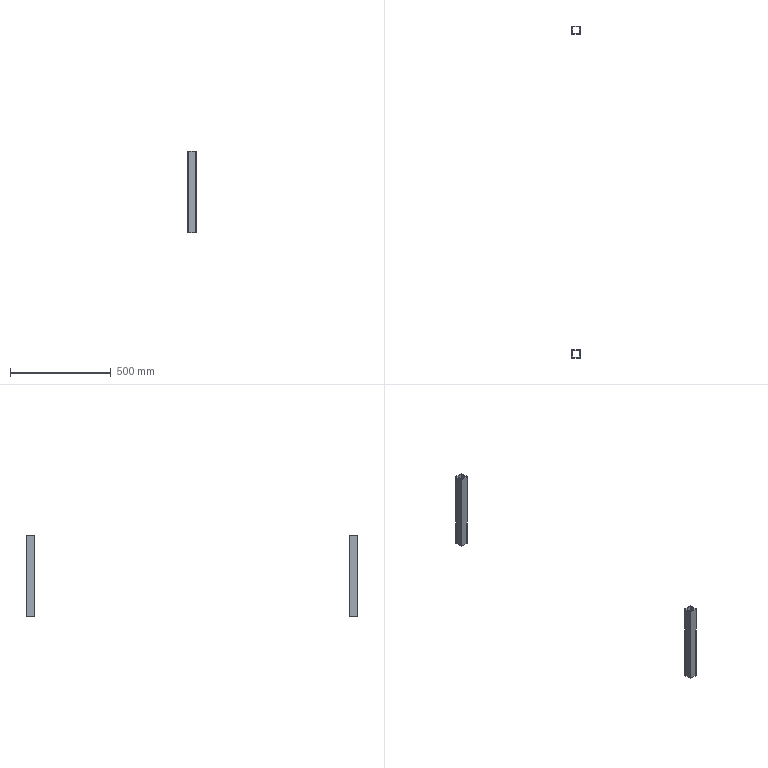Part | STEP file | ASND-0110-E63-HLTP01标准Lower机架-05 | 2 solids | 20 faces | box 40 x 1650 x 405 mm | volume 466560 mm3 | plane 20
STEP:
#1=CARTESIAN_POINT('',(0.,0.,0.));
#2=DIRECTION('',(0.,0.,1.));
#3=DIRECTION('',(1.,0.,0.));
#4=AXIS2_PLACEMENT_3D('',#1,#2,#3);
#5=CARTESIAN_POINT('',(660.,0.,405.));
#6=VERTEX_POINT('',#5);
#7=CARTESIAN_POINT('',(620.,0.,405.));
#8=VERTEX_POINT('',#7);
#9=CARTESIAN_POINT('',(660.,0.,405.));
#10=DIRECTION('',(-1.,0.,0.));
#11=VECTOR('',#10,1.);
#12=LINE('',#9,#11);
#13=CARTESIAN_POINT('',(620.,0.,461.569));
#14=DIRECTION('',(0.,-1.,0.));
#15=DIRECTION('',(0.7071,0.,0.7071));
#16=AXIS2_PLACEMENT_3D('',#13,#14,#15);
#17=PLANE('',#16);
#18=CARTESIAN_POINT('',(-11.716,-68.284));
#19=DIRECTION('',(-0.7071,0.7071));
#20=VECTOR('',#19,1.);
#21=LINE('',#18,#20);
#22=(GEOMETRIC_REPRESENTATION_CONTEXT(2)PARAMETRIC_REPRESENTATION_CONTEXT()REPRESENTATION_CONTEXT('',''));
#23=DEFINITIONAL_REPRESENTATION('',(#21),#22);
#24=PCURVE('',#17,#23);
#25=CARTESIAN_POINT('',(1364.853,-1650.,405.));
#26=DIRECTION('',(0.,0.,1.));
#27=DIRECTION('',(0.7071,0.7071,0.));
#28=AXIS2_PLACEMENT_3D('',#25,#26,#27);
#29=PLANE('',#28);
#30=CARTESIAN_POINT('',(668.32,1665.132));
#31=DIRECTION('',(-0.7071,0.7071));
#32=VECTOR('',#31,1.);
#33=LINE('',#30,#32);
#34=(GEOMETRIC_REPRESENTATION_CONTEXT(2)PARAMETRIC_REPRESENTATION_CONTEXT()REPRESENTATION_CONTEXT('',''));
#35=DEFINITIONAL_REPRESENTATION('',(#33),#34);
#36=PCURVE('',#29,#35);
#37=SURFACE_CURVE('',#12,(#24,#36),.PCURVE_S1.);
#38=EDGE_CURVE('',#6,#8,#37,.T.);
#39=ORIENTED_EDGE('',*,*,#38,.F.);
#40=CARTESIAN_POINT('',(660.,0.,0.));
#41=VERTEX_POINT('',#40);
#42=CARTESIAN_POINT('',(660.,0.,405.));
#43=DIRECTION('',(0.,0.,-1.));
#44=VECTOR('',#43,1.);
#45=LINE('',#42,#44);
#46=CARTESIAN_POINT('',(-11.716,-68.284));
#47=DIRECTION('',(-0.7071,-0.7071));
#48=VECTOR('',#47,1.);
#49=LINE('',#46,#48);
#50=(GEOMETRIC_REPRESENTATION_CONTEXT(2)PARAMETRIC_REPRESENTATION_CONTEXT()REPRESENTATION_CONTEXT('',''));
#51=DEFINITIONAL_REPRESENTATION('',(#49),#50);
#52=PCURVE('',#17,#51);
#53=CARTESIAN_POINT('',(660.,-40.,461.569));
#54=DIRECTION('',(-1.,0.,0.));
#55=DIRECTION('',(0.,0.7071,0.7071));
#56=AXIS2_PLACEMENT_3D('',#53,#54,#55);
#57=PLANE('',#56);
#58=CARTESIAN_POINT('',(-11.716,68.284));
#59=DIRECTION('',(-0.7071,0.7071));
#60=VECTOR('',#59,1.);
#61=LINE('',#58,#60);
#62=(GEOMETRIC_REPRESENTATION_CONTEXT(2)PARAMETRIC_REPRESENTATION_CONTEXT()REPRESENTATION_CONTEXT('',''));
#63=DEFINITIONAL_REPRESENTATION('',(#61),#62);
#64=PCURVE('',#57,#63);
#65=SURFACE_CURVE('',#45,(#52,#64),.PCURVE_S1.);
#66=EDGE_CURVE('',#6,#41,#65,.T.);
#67=ORIENTED_EDGE('',*,*,#66,.T.);
#68=CARTESIAN_POINT('',(620.,0.,0.));
#69=VERTEX_POINT('',#68);
#70=CARTESIAN_POINT('',(660.,0.,0.));
#71=DIRECTION('',(-1.,0.,0.));
#72=VECTOR('',#71,1.);
#73=LINE('',#70,#72);
#74=CARTESIAN_POINT('',(-298.094,-354.663));
#75=DIRECTION('',(-0.7071,0.7071));
#76=VECTOR('',#75,1.);
#77=LINE('',#74,#76);
#78=(GEOMETRIC_REPRESENTATION_CONTEXT(2)PARAMETRIC_REPRESENTATION_CONTEXT()REPRESENTATION_CONTEXT('',''));
#79=DEFINITIONAL_REPRESENTATION('',(#77),#78);
#80=PCURVE('',#17,#79);
#81=CARTESIAN_POINT('',(0.,0.,0.));
#82=DIRECTION('',(0.,0.,-1.));
#83=DIRECTION('',(0.7071,0.7071,0.));
#84=AXIS2_PLACEMENT_3D('',#81,#82,#83);
#85=PLANE('',#84);
#86=CARTESIAN_POINT('',(466.69,466.69));
#87=DIRECTION('',(-0.7071,-0.7071));
#88=VECTOR('',#87,1.);
#89=LINE('',#86,#88);
#90=(GEOMETRIC_REPRESENTATION_CONTEXT(2)PARAMETRIC_REPRESENTATION_CONTEXT()REPRESENTATION_CONTEXT('',''));
#91=DEFINITIONAL_REPRESENTATION('',(#89),#90);
#92=PCURVE('',#85,#91);
#93=SURFACE_CURVE('',#73,(#80,#92),.PCURVE_S1.);
#94=EDGE_CURVE('',#41,#69,#93,.T.);
#95=ORIENTED_EDGE('',*,*,#94,.T.);
#96=CARTESIAN_POINT('',(620.,0.,405.));
#97=DIRECTION('',(0.,0.,-1.));
#98=VECTOR('',#97,1.);
#99=LINE('',#96,#98);
#100=CARTESIAN_POINT('',(-40.,-40.));
#101=DIRECTION('',(-0.7071,-0.7071));
#102=VECTOR('',#101,1.);
#103=LINE('',#100,#102);
#104=(GEOMETRIC_REPRESENTATION_CONTEXT(2)PARAMETRIC_REPRESENTATION_CONTEXT()REPRESENTATION_CONTEXT('',''));
#105=DEFINITIONAL_REPRESENTATION('',(#103),#104);
#106=PCURVE('',#17,#105);
#107=CARTESIAN_POINT('',(620.,-40.,461.569));
#108=DIRECTION('',(1.,0.,0.));
#109=DIRECTION('',(0.,0.7071,0.7071));
#110=AXIS2_PLACEMENT_3D('',#107,#108,#109);
#111=PLANE('',#110);
#112=CARTESIAN_POINT('',(-11.716,-68.284));
#113=DIRECTION('',(-0.7071,-0.7071));
#114=VECTOR('',#113,1.);
#115=LINE('',#112,#114);
#116=(GEOMETRIC_REPRESENTATION_CONTEXT(2)PARAMETRIC_REPRESENTATION_CONTEXT()REPRESENTATION_CONTEXT('',''));
#117=DEFINITIONAL_REPRESENTATION('',(#115),#116);
#118=PCURVE('',#111,#117);
#119=SURFACE_CURVE('',#99,(#106,#118),.PCURVE_S1.);
#120=EDGE_CURVE('',#8,#69,#119,.T.);
#121=ORIENTED_EDGE('',*,*,#120,.F.);
#122=EDGE_LOOP('',(#39,#67,#95,#121));
#123=FACE_BOUND('',#122,.T.);
#124=ADVANCED_FACE('',(#123),#17,.F.);
#125=CARTESIAN_POINT('',(660.,-40.,405.));
#126=VERTEX_POINT('',#125);
#127=CARTESIAN_POINT('',(660.,-40.,405.));
#128=DIRECTION('',(0.,1.,0.));
#129=VECTOR('',#128,1.);
#130=LINE('',#127,#129);
#131=CARTESIAN_POINT('',(-40.,40.));
#132=DIRECTION('',(0.7071,0.7071));
#133=VECTOR('',#132,1.);
#134=LINE('',#131,#133);
#135=(GEOMETRIC_REPRESENTATION_CONTEXT(2)PARAMETRIC_REPRESENTATION_CONTEXT()REPRESENTATION_CONTEXT('',''));
#136=DEFINITIONAL_REPRESENTATION('',(#134),#135);
#137=PCURVE('',#57,#136);
#138=CARTESIAN_POINT('',(640.036,1636.848));
#139=DIRECTION('',(0.7071,0.7071));
#140=VECTOR('',#139,1.);
#141=LINE('',#138,#140);
#142=(GEOMETRIC_REPRESENTATION_CONTEXT(2)PARAMETRIC_REPRESENTATION_CONTEXT()REPRESENTATION_CONTEXT('',''));
#143=DEFINITIONAL_REPRESENTATION('',(#141),#142);
#144=PCURVE('',#29,#143);
#145=SURFACE_CURVE('',#130,(#137,#144),.PCURVE_S1.);
#146=EDGE_CURVE('',#126,#6,#145,.T.);
#147=ORIENTED_EDGE('',*,*,#146,.F.);
#148=CARTESIAN_POINT('',(660.,-40.,0.));
#149=VERTEX_POINT('',#148);
#150=CARTESIAN_POINT('',(660.,-40.,405.));
#151=DIRECTION('',(0.,0.,-1.));
#152=VECTOR('',#151,1.);
#153=LINE('',#150,#152);
#154=CARTESIAN_POINT('',(-40.,40.));
#155=DIRECTION('',(-0.7071,0.7071));
#156=VECTOR('',#155,1.);
#157=LINE('',#154,#156);
#158=(GEOMETRIC_REPRESENTATION_CONTEXT(2)PARAMETRIC_REPRESENTATION_CONTEXT()REPRESENTATION_CONTEXT('',''));
#159=DEFINITIONAL_REPRESENTATION('',(#157),#158);
#160=PCURVE('',#57,#159);
#161=CARTESIAN_POINT('',(620.,-40.,461.569));
#162=DIRECTION('',(0.,1.,0.));
#163=DIRECTION('',(0.7071,0.,0.7071));
#164=AXIS2_PLACEMENT_3D('',#161,#162,#163);
#165=PLANE('',#164);
#166=CARTESIAN_POINT('',(-11.716,68.284));
#167=DIRECTION('',(-0.7071,0.7071));
#168=VECTOR('',#167,1.);
#169=LINE('',#166,#168);
#170=(GEOMETRIC_REPRESENTATION_CONTEXT(2)PARAMETRIC_REPRESENTATION_CONTEXT()REPRESENTATION_CONTEXT('',''));
#171=DEFINITIONAL_REPRESENTATION('',(#169),#170);
#172=PCURVE('',#165,#171);
#173=SURFACE_CURVE('',#153,(#160,#172),.PCURVE_S1.);
#174=EDGE_CURVE('',#126,#149,#173,.T.);
#175=ORIENTED_EDGE('',*,*,#174,.T.);
#176=CARTESIAN_POINT('',(660.,-40.,0.));
#177=DIRECTION('',(0.,1.,0.));
#178=VECTOR('',#177,1.);
#179=LINE('',#176,#178);
#180=CARTESIAN_POINT('',(-326.378,326.378));
#181=DIRECTION('',(0.7071,0.7071));
#182=VECTOR('',#181,1.);
#183=LINE('',#180,#182);
#184=(GEOMETRIC_REPRESENTATION_CONTEXT(2)PARAMETRIC_REPRESENTATION_CONTEXT()REPRESENTATION_CONTEXT('',''));
#185=DEFINITIONAL_REPRESENTATION('',(#183),#184);
#186=PCURVE('',#57,#185);
#187=CARTESIAN_POINT('',(438.406,494.975));
#188=DIRECTION('',(0.7071,-0.7071));
#189=VECTOR('',#188,1.);
#190=LINE('',#187,#189);
#191=(GEOMETRIC_REPRESENTATION_CONTEXT(2)PARAMETRIC_REPRESENTATION_CONTEXT()REPRESENTATION_CONTEXT('',''));
#192=DEFINITIONAL_REPRESENTATION('',(#190),#191);
#193=PCURVE('',#85,#192);
#194=SURFACE_CURVE('',#179,(#186,#193),.PCURVE_S1.);
#195=EDGE_CURVE('',#149,#41,#194,.T.);
#196=ORIENTED_EDGE('',*,*,#195,.T.);
#197=ORIENTED_EDGE('',*,*,#66,.F.);
#198=EDGE_LOOP('',(#147,#175,#196,#197));
#199=FACE_BOUND('',#198,.T.);
#200=ADVANCED_FACE('',(#199),#57,.F.);
#201=CARTESIAN_POINT('',(620.,-40.,405.));
#202=VERTEX_POINT('',#201);
#203=CARTESIAN_POINT('',(620.,-40.,405.));
#204=DIRECTION('',(1.,0.,0.));
#205=VECTOR('',#204,1.);
#206=LINE('',#203,#205);
#207=CARTESIAN_POINT('',(-40.,40.));
#208=DIRECTION('',(0.7071,0.7071));
#209=VECTOR('',#208,1.);
#210=LINE('',#207,#209);
#211=(GEOMETRIC_REPRESENTATION_CONTEXT(2)PARAMETRIC_REPRESENTATION_CONTEXT()REPRESENTATION_CONTEXT('',''));
#212=DEFINITIONAL_REPRESENTATION('',(#210),#211);
#213=PCURVE('',#165,#212);
#214=CARTESIAN_POINT('',(611.751,1665.132));
#215=DIRECTION('',(0.7071,-0.7071));
#216=VECTOR('',#215,1.);
#217=LINE('',#214,#216);
#218=(GEOMETRIC_REPRESENTATION_CONTEXT(2)PARAMETRIC_REPRESENTATION_CONTEXT()REPRESENTATION_CONTEXT('',''));
#219=DEFINITIONAL_REPRESENTATION('',(#217),#218);
#220=PCURVE('',#29,#219);
#221=SURFACE_CURVE('',#206,(#213,#220),.PCURVE_S1.);
#222=EDGE_CURVE('',#202,#126,#221,.T.);
#223=ORIENTED_EDGE('',*,*,#222,.F.);
#224=CARTESIAN_POINT('',(620.,-40.,0.));
#225=VERTEX_POINT('',#224);
#226=CARTESIAN_POINT('',(620.,-40.,405.));
#227=DIRECTION('',(0.,0.,-1.));
#228=VECTOR('',#227,1.);
#229=LINE('',#226,#228);
#230=CARTESIAN_POINT('',(-40.,40.));
#231=DIRECTION('',(-0.7071,0.7071));
#232=VECTOR('',#231,1.);
#233=LINE('',#230,#232);
#234=(GEOMETRIC_REPRESENTATION_CONTEXT(2)PARAMETRIC_REPRESENTATION_CONTEXT()REPRESENTATION_CONTEXT('',''));
#235=DEFINITIONAL_REPRESENTATION('',(#233),#234);
#236=PCURVE('',#165,#235);
#237=CARTESIAN_POINT('',(-40.,-40.));
#238=DIRECTION('',(-0.7071,-0.7071));
#239=VECTOR('',#238,1.);
#240=LINE('',#237,#239);
#241=(GEOMETRIC_REPRESENTATION_CONTEXT(2)PARAMETRIC_REPRESENTATION_CONTEXT()REPRESENTATION_CONTEXT('',''));
#242=DEFINITIONAL_REPRESENTATION('',(#240),#241);
#243=PCURVE('',#111,#242);
#244=SURFACE_CURVE('',#229,(#236,#243),.PCURVE_S1.);
#245=EDGE_CURVE('',#202,#225,#244,.T.);
#246=ORIENTED_EDGE('',*,*,#245,.T.);
#247=CARTESIAN_POINT('',(620.,-40.,0.));
#248=DIRECTION('',(1.,0.,0.));
#249=VECTOR('',#248,1.);
#250=LINE('',#247,#249);
#251=CARTESIAN_POINT('',(-326.378,326.378));
#252=DIRECTION('',(0.7071,0.7071));
#253=VECTOR('',#252,1.);
#254=LINE('',#251,#253);
#255=(GEOMETRIC_REPRESENTATION_CONTEXT(2)PARAMETRIC_REPRESENTATION_CONTEXT()REPRESENTATION_CONTEXT('',''));
#256=DEFINITIONAL_REPRESENTATION('',(#254),#255);
#257=PCURVE('',#165,#256);
#258=CARTESIAN_POINT('',(410.122,466.69));
#259=DIRECTION('',(0.7071,0.7071));
#260=VECTOR('',#259,1.);
#261=LINE('',#258,#260);
#262=(GEOMETRIC_REPRESENTATION_CONTEXT(2)PARAMETRIC_REPRESENTATION_CONTEXT()REPRESENTATION_CONTEXT('',''));
#263=DEFINITIONAL_REPRESENTATION('',(#261),#262);
#264=PCURVE('',#85,#263);
#265=SURFACE_CURVE('',#250,(#257,#264),.PCURVE_S1.);
#266=EDGE_CURVE('',#225,#149,#265,.T.);
#267=ORIENTED_EDGE('',*,*,#266,.T.);
#268=ORIENTED_EDGE('',*,*,#174,.F.);
#269=EDGE_LOOP('',(#223,#246,#267,#268));
#270=FACE_BOUND('',#269,.T.);
#271=ADVANCED_FACE('',(#270),#165,.F.);
#272=CARTESIAN_POINT('',(620.,0.,405.));
#273=DIRECTION('',(0.,-1.,0.));
#274=VECTOR('',#273,1.);
#275=LINE('',#272,#274);
#276=CARTESIAN_POINT('',(-11.716,-68.284));
#277=DIRECTION('',(-0.7071,0.7071));
#278=VECTOR('',#277,1.);
#279=LINE('',#276,#278);
#280=(GEOMETRIC_REPRESENTATION_CONTEXT(2)PARAMETRIC_REPRESENTATION_CONTEXT()REPRESENTATION_CONTEXT('',''));
#281=DEFINITIONAL_REPRESENTATION('',(#279),#280);
#282=PCURVE('',#111,#281);
#283=CARTESIAN_POINT('',(640.036,1693.417));
#284=DIRECTION('',(-0.7071,-0.7071));
#285=VECTOR('',#284,1.);
#286=LINE('',#283,#285);
#287=(GEOMETRIC_REPRESENTATION_CONTEXT(2)PARAMETRIC_REPRESENTATION_CONTEXT()REPRESENTATION_CONTEXT('',''));
#288=DEFINITIONAL_REPRESENTATION('',(#286),#287);
#289=PCURVE('',#29,#288);
#290=SURFACE_CURVE('',#275,(#282,#289),.PCURVE_S1.);
#291=EDGE_CURVE('',#8,#202,#290,.T.);
#292=ORIENTED_EDGE('',*,*,#291,.F.);
#293=ORIENTED_EDGE('',*,*,#120,.T.);
#294=CARTESIAN_POINT('',(620.,0.,0.));
#295=DIRECTION('',(0.,-1.,0.));
#296=VECTOR('',#295,1.);
#297=LINE('',#294,#296);
#298=CARTESIAN_POINT('',(-298.094,-354.663));
#299=DIRECTION('',(-0.7071,0.7071));
#300=VECTOR('',#299,1.);
#301=LINE('',#298,#300);
#302=(GEOMETRIC_REPRESENTATION_CONTEXT(2)PARAMETRIC_REPRESENTATION_CONTEXT()REPRESENTATION_CONTEXT('',''));
#303=DEFINITIONAL_REPRESENTATION('',(#301),#302);
#304=PCURVE('',#111,#303);
#305=CARTESIAN_POINT('',(438.406,438.406));
#306=DIRECTION('',(-0.7071,0.7071));
#307=VECTOR('',#306,1.);
#308=LINE('',#305,#307);
#309=(GEOMETRIC_REPRESENTATION_CONTEXT(2)PARAMETRIC_REPRESENTATION_CONTEXT()REPRESENTATION_CONTEXT('',''));
#310=DEFINITIONAL_REPRESENTATION('',(#308),#309);
#311=PCURVE('',#85,#310);
#312=SURFACE_CURVE('',#297,(#304,#311),.PCURVE_S1.);
#313=EDGE_CURVE('',#69,#225,#312,.T.);
#314=ORIENTED_EDGE('',*,*,#313,.T.);
#315=ORIENTED_EDGE('',*,*,#245,.F.);
#316=EDGE_LOOP('',(#292,#293,#314,#315));
#317=FACE_BOUND('',#316,.T.);
#318=ADVANCED_FACE('',(#317),#111,.F.);
#319=ORIENTED_EDGE('',*,*,#313,.F.);
#320=ORIENTED_EDGE('',*,*,#94,.F.);
#321=ORIENTED_EDGE('',*,*,#195,.F.);
#322=ORIENTED_EDGE('',*,*,#266,.F.);
#323=EDGE_LOOP('',(#319,#320,#321,#322));
#324=FACE_BOUND('',#323,.T.);
#325=CARTESIAN_POINT('',(656.,-4.,0.));
#326=VERTEX_POINT('',#325);
#327=CARTESIAN_POINT('',(624.,-4.,0.));
#328=VERTEX_POINT('',#327);
#329=CARTESIAN_POINT('',(656.,-4.,0.));
#330=DIRECTION('',(-1.,0.,0.));
#331=VECTOR('',#330,1.);
#332=LINE('',#329,#331);
#333=CARTESIAN_POINT('',(461.034,466.69));
#334=DIRECTION('',(-0.7071,-0.7071));
#335=VECTOR('',#334,1.);
#336=LINE('',#333,#335);
#337=(GEOMETRIC_REPRESENTATION_CONTEXT(2)PARAMETRIC_REPRESENTATION_CONTEXT()REPRESENTATION_CONTEXT('',''));
#338=DEFINITIONAL_REPRESENTATION('',(#336),#337);
#339=PCURVE('',#85,#338);
#340=CARTESIAN_POINT('',(624.,-4.,461.569));
#341=DIRECTION('',(0.,-1.,0.));
#342=DIRECTION('',(0.7071,0.,0.7071));
#343=AXIS2_PLACEMENT_3D('',#340,#341,#342);
#344=PLANE('',#343);
#345=CARTESIAN_POINT('',(-303.751,-349.006));
#346=DIRECTION('',(-0.7071,0.7071));
#347=VECTOR('',#346,1.);
#348=LINE('',#345,#347);
#349=(GEOMETRIC_REPRESENTATION_CONTEXT(2)PARAMETRIC_REPRESENTATION_CONTEXT()REPRESENTATION_CONTEXT('',''));
#350=DEFINITIONAL_REPRESENTATION('',(#348),#349);
#351=PCURVE('',#344,#350);
#352=SURFACE_CURVE('',#332,(#339,#351),.PCURVE_S1.);
#353=EDGE_CURVE('',#326,#328,#352,.T.);
#354=ORIENTED_EDGE('',*,*,#353,.T.);
#355=CARTESIAN_POINT('',(624.,-36.,0.));
#356=VERTEX_POINT('',#355);
#357=CARTESIAN_POINT('',(624.,-4.,0.));
#358=DIRECTION('',(0.,-1.,0.));
#359=VECTOR('',#358,1.);
#360=LINE('',#357,#359);
#361=CARTESIAN_POINT('',(438.406,444.063));
#362=DIRECTION('',(-0.7071,0.7071));
#363=VECTOR('',#362,1.);
#364=LINE('',#361,#363);
#365=(GEOMETRIC_REPRESENTATION_CONTEXT(2)PARAMETRIC_REPRESENTATION_CONTEXT()REPRESENTATION_CONTEXT('',''));
#366=DEFINITIONAL_REPRESENTATION('',(#364),#365);
#367=PCURVE('',#85,#366);
#368=CARTESIAN_POINT('',(624.,-36.,461.569));
#369=DIRECTION('',(1.,0.,0.));
#370=DIRECTION('',(0.,0.7071,0.7071));
#371=AXIS2_PLACEMENT_3D('',#368,#369,#370);
#372=PLANE('',#371);
#373=CARTESIAN_POINT('',(-303.751,-349.006));
#374=DIRECTION('',(-0.7071,0.7071));
#375=VECTOR('',#374,1.);
#376=LINE('',#373,#375);
#377=(GEOMETRIC_REPRESENTATION_CONTEXT(2)PARAMETRIC_REPRESENTATION_CONTEXT()REPRESENTATION_CONTEXT('',''));
#378=DEFINITIONAL_REPRESENTATION('',(#376),#377);
#379=PCURVE('',#372,#378);
#380=SURFACE_CURVE('',#360,(#367,#379),.PCURVE_S1.);
#381=EDGE_CURVE('',#328,#356,#380,.T.);
#382=ORIENTED_EDGE('',*,*,#381,.T.);
#383=CARTESIAN_POINT('',(656.,-36.,0.));
#384=VERTEX_POINT('',#383);
#385=CARTESIAN_POINT('',(624.,-36.,0.));
#386=DIRECTION('',(1.,0.,0.));
#387=VECTOR('',#386,1.);
#388=LINE('',#385,#387);
#389=CARTESIAN_POINT('',(415.779,466.69));
#390=DIRECTION('',(0.7071,0.7071));
#391=VECTOR('',#390,1.);
#392=LINE('',#389,#391);
#393=(GEOMETRIC_REPRESENTATION_CONTEXT(2)PARAMETRIC_REPRESENTATION_CONTEXT()REPRESENTATION_CONTEXT('',''));
#394=DEFINITIONAL_REPRESENTATION('',(#392),#393);
#395=PCURVE('',#85,#394);
#396=CARTESIAN_POINT('',(624.,-36.,461.569));
#397=DIRECTION('',(0.,1.,0.));
#398=DIRECTION('',(0.7071,0.,0.7071));
#399=AXIS2_PLACEMENT_3D('',#396,#397,#398);
#400=PLANE('',#399);
#401=CARTESIAN_POINT('',(-326.378,326.378));
#402=DIRECTION('',(0.7071,0.7071));
#403=VECTOR('',#402,1.);
#404=LINE('',#401,#403);
#405=(GEOMETRIC_REPRESENTATION_CONTEXT(2)PARAMETRIC_REPRESENTATION_CONTEXT()REPRESENTATION_CONTEXT('',''));
#406=DEFINITIONAL_REPRESENTATION('',(#404),#405);
#407=PCURVE('',#400,#406);
#408=SURFACE_CURVE('',#388,(#395,#407),.PCURVE_S1.);
#409=EDGE_CURVE('',#356,#384,#408,.T.);
#410=ORIENTED_EDGE('',*,*,#409,.T.);
#411=CARTESIAN_POINT('',(656.,-36.,0.));
#412=DIRECTION('',(0.,1.,0.));
#413=VECTOR('',#412,1.);
#414=LINE('',#411,#413);
#415=CARTESIAN_POINT('',(438.406,489.318));
#416=DIRECTION('',(0.7071,-0.7071));
#417=VECTOR('',#416,1.);
#418=LINE('',#415,#417);
#419=(GEOMETRIC_REPRESENTATION_CONTEXT(2)PARAMETRIC_REPRESENTATION_CONTEXT()REPRESENTATION_CONTEXT('',''));
#420=DEFINITIONAL_REPRESENTATION('',(#418),#419);
#421=PCURVE('',#85,#420);
#422=CARTESIAN_POINT('',(656.,-36.,461.569));
#423=DIRECTION('',(-1.,0.,0.));
#424=DIRECTION('',(0.,0.7071,0.7071));
#425=AXIS2_PLACEMENT_3D('',#422,#423,#424);
#426=PLANE('',#425);
#427=CARTESIAN_POINT('',(-326.378,326.378));
#428=DIRECTION('',(0.7071,0.7071));
#429=VECTOR('',#428,1.);
#430=LINE('',#427,#429);
#431=(GEOMETRIC_REPRESENTATION_CONTEXT(2)PARAMETRIC_REPRESENTATION_CONTEXT()REPRESENTATION_CONTEXT('',''));
#432=DEFINITIONAL_REPRESENTATION('',(#430),#431);
#433=PCURVE('',#426,#432);
#434=SURFACE_CURVE('',#414,(#421,#433),.PCURVE_S1.);
#435=EDGE_CURVE('',#384,#326,#434,.T.);
#436=ORIENTED_EDGE('',*,*,#435,.T.);
#437=EDGE_LOOP('',(#354,#382,#410,#436));
#438=FACE_BOUND('',#437,.T.);
#439=ADVANCED_FACE('',(#324,#438),#85,.T.);
#440=CARTESIAN_POINT('',(656.,-4.,405.));
#441=VERTEX_POINT('',#440);
#442=CARTESIAN_POINT('',(656.,-4.,405.));
#443=DIRECTION('',(0.,0.,-1.));
#444=VECTOR('',#443,1.);
#445=LINE('',#442,#444);
#446=CARTESIAN_POINT('',(-17.373,-62.627));
#447=DIRECTION('',(-0.7071,-0.7071));
#448=VECTOR('',#447,1.);
#449=LINE('',#446,#448);
#450=(GEOMETRIC_REPRESENTATION_CONTEXT(2)PARAMETRIC_REPRESENTATION_CONTEXT()REPRESENTATION_CONTEXT('',''));
#451=DEFINITIONAL_REPRESENTATION('',(#449),#450);
#452=PCURVE('',#344,#451);
#453=CARTESIAN_POINT('',(-17.373,62.627));
#454=DIRECTION('',(-0.7071,0.7071));
#455=VECTOR('',#454,1.);
#456=LINE('',#453,#455);
#457=(GEOMETRIC_REPRESENTATION_CONTEXT(2)PARAMETRIC_REPRESENTATION_CONTEXT()REPRESENTATION_CONTEXT('',''));
#458=DEFINITIONAL_REPRESENTATION('',(#456),#457);
#459=PCURVE('',#426,#458);
#460=SURFACE_CURVE('',#445,(#452,#459),.PCURVE_S1.);
#461=EDGE_CURVE('',#441,#326,#460,.T.);
#462=ORIENTED_EDGE('',*,*,#461,.F.);
#463=CARTESIAN_POINT('',(624.,-4.,405.));
#464=VERTEX_POINT('',#463);
#465=CARTESIAN_POINT('',(656.,-4.,405.));
#466=DIRECTION('',(-1.,0.,0.));
#467=VECTOR('',#466,1.);
#468=LINE('',#465,#467);
#469=CARTESIAN_POINT('',(-17.373,-62.627));
#470=DIRECTION('',(-0.7071,0.7071));
#471=VECTOR('',#470,1.);
#472=LINE('',#469,#471);
#473=(GEOMETRIC_REPRESENTATION_CONTEXT(2)PARAMETRIC_REPRESENTATION_CONTEXT()REPRESENTATION_CONTEXT('',''));
#474=DEFINITIONAL_REPRESENTATION('',(#472),#473);
#475=PCURVE('',#344,#474);
#476=CARTESIAN_POINT('',(662.663,1665.132));
#477=DIRECTION('',(-0.7071,0.7071));
#478=VECTOR('',#477,1.);
#479=LINE('',#476,#478);
#480=(GEOMETRIC_REPRESENTATION_CONTEXT(2)PARAMETRIC_REPRESENTATION_CONTEXT()REPRESENTATION_CONTEXT('',''));
#481=DEFINITIONAL_REPRESENTATION('',(#479),#480);
#482=PCURVE('',#29,#481);
#483=SURFACE_CURVE('',#468,(#475,#482),.PCURVE_S1.);
#484=EDGE_CURVE('',#441,#464,#483,.T.);
#485=ORIENTED_EDGE('',*,*,#484,.T.);
#486=CARTESIAN_POINT('',(624.,-4.,405.));
#487=DIRECTION('',(0.,0.,-1.));
#488=VECTOR('',#487,1.);
#489=LINE('',#486,#488);
#490=CARTESIAN_POINT('',(-40.,-40.));
#491=DIRECTION('',(-0.7071,-0.7071));
#492=VECTOR('',#491,1.);
#493=LINE('',#490,#492);
#494=(GEOMETRIC_REPRESENTATION_CONTEXT(2)PARAMETRIC_REPRESENTATION_CONTEXT()REPRESENTATION_CONTEXT('',''));
#495=DEFINITIONAL_REPRESENTATION('',(#493),#494);
#496=PCURVE('',#344,#495);
#497=CARTESIAN_POINT('',(-17.373,-62.627));
#498=DIRECTION('',(-0.7071,-0.7071));
#499=VECTOR('',#498,1.);
#500=LINE('',#497,#499);
#501=(GEOMETRIC_REPRESENTATION_CONTEXT(2)PARAMETRIC_REPRESENTATION_CONTEXT()REPRESENTATION_CONTEXT('',''));
#502=DEFINITIONAL_REPRESENTATION('',(#500),#501);
#503=PCURVE('',#372,#502);
#504=SURFACE_CURVE('',#489,(#496,#503),.PCURVE_S1.);
#505=EDGE_CURVE('',#464,#328,#504,.T.);
#506=ORIENTED_EDGE('',*,*,#505,.T.);
#507=ORIENTED_EDGE('',*,*,#353,.F.);
#508=EDGE_LOOP('',(#462,#485,#506,#507));
#509=FACE_BOUND('',#508,.T.);
#510=ADVANCED_FACE('',(#509),#344,.T.);
#511=CARTESIAN_POINT('',(656.,-36.,405.));
#512=VERTEX_POINT('',#511);
#513=CARTESIAN_POINT('',(656.,-36.,405.));
#514=DIRECTION('',(0.,0.,-1.));
#515=VECTOR('',#514,1.);
#516=LINE('',#513,#515);
#517=CARTESIAN_POINT('',(-40.,40.));
#518=DIRECTION('',(-0.7071,0.7071));
#519=VECTOR('',#518,1.);
#520=LINE('',#517,#519);
#521=(GEOMETRIC_REPRESENTATION_CONTEXT(2)PARAMETRIC_REPRESENTATION_CONTEXT()REPRESENTATION_CONTEXT('',''));
#522=DEFINITIONAL_REPRESENTATION('',(#520),#521);
#523=PCURVE('',#426,#522);
#524=CARTESIAN_POINT('',(-17.373,62.627));
#525=DIRECTION('',(-0.7071,0.7071));
#526=VECTOR('',#525,1.);
#527=LINE('',#524,#526);
#528=(GEOMETRIC_REPRESENTATION_CONTEXT(2)PARAMETRIC_REPRESENTATION_CONTEXT()REPRESENTATION_CONTEXT('',''));
#529=DEFINITIONAL_REPRESENTATION('',(#527),#528);
#530=PCURVE('',#400,#529);
#531=SURFACE_CURVE('',#516,(#523,#530),.PCURVE_S1.);
#532=EDGE_CURVE('',#512,#384,#531,.T.);
#533=ORIENTED_EDGE('',*,*,#532,.F.);
#534=CARTESIAN_POINT('',(656.,-36.,405.));
#535=DIRECTION('',(0.,1.,0.));
#536=VECTOR('',#535,1.);
#537=LINE('',#534,#536);
#538=CARTESIAN_POINT('',(-40.,40.));
#539=DIRECTION('',(0.7071,0.7071));
#540=VECTOR('',#539,1.);
#541=LINE('',#538,#540);
#542=(GEOMETRIC_REPRESENTATION_CONTEXT(2)PARAMETRIC_REPRESENTATION_CONTEXT()REPRESENTATION_CONTEXT('',''));
#543=DEFINITIONAL_REPRESENTATION('',(#541),#542);
#544=PCURVE('',#426,#543);
#545=CARTESIAN_POINT('',(640.036,1642.505));
#546=DIRECTION('',(0.7071,0.7071));
#547=VECTOR('',#546,1.);
#548=LINE('',#545,#547);
#549=(GEOMETRIC_REPRESENTATION_CONTEXT(2)PARAMETRIC_REPRESENTATION_CONTEXT()REPRESENTATION_CONTEXT('',''));
#550=DEFINITIONAL_REPRESENTATION('',(#548),#549);
#551=PCURVE('',#29,#550);
#552=SURFACE_CURVE('',#537,(#544,#551),.PCURVE_S1.);
#553=EDGE_CURVE('',#512,#441,#552,.T.);
#554=ORIENTED_EDGE('',*,*,#553,.T.);
#555=ORIENTED_EDGE('',*,*,#461,.T.);
#556=ORIENTED_EDGE('',*,*,#435,.F.);
#557=EDGE_LOOP('',(#533,#554,#555,#556));
#558=FACE_BOUND('',#557,.T.);
#559=ADVANCED_FACE('',(#558),#426,.T.);
#560=CARTESIAN_POINT('',(624.,-36.,405.));
#561=VERTEX_POINT('',#560);
#562=CARTESIAN_POINT('',(624.,-36.,405.));
#563=DIRECTION('',(0.,0.,-1.));
#564=VECTOR('',#563,1.);
#565=LINE('',#562,#564);
#566=CARTESIAN_POINT('',(-40.,40.));
#567=DIRECTION('',(-0.7071,0.7071));
#568=VECTOR('',#567,1.);
#569=LINE('',#566,#568);
#570=(GEOMETRIC_REPRESENTATION_CONTEXT(2)PARAMETRIC_REPRESENTATION_CONTEXT()REPRESENTATION_CONTEXT('',''));
#571=DEFINITIONAL_REPRESENTATION('',(#569),#570);
#572=PCURVE('',#400,#571);
#573=CARTESIAN_POINT('',(-40.,-40.));
#574=DIRECTION('',(-0.7071,-0.7071));
#575=VECTOR('',#574,1.);
#576=LINE('',#573,#575);
#577=(GEOMETRIC_REPRESENTATION_CONTEXT(2)PARAMETRIC_REPRESENTATION_CONTEXT()REPRESENTATION_CONTEXT('',''));
#578=DEFINITIONAL_REPRESENTATION('',(#576),#577);
#579=PCURVE('',#372,#578);
#580=SURFACE_CURVE('',#565,(#572,#579),.PCURVE_S1.);
#581=EDGE_CURVE('',#561,#356,#580,.T.);
#582=ORIENTED_EDGE('',*,*,#581,.F.);
#583=CARTESIAN_POINT('',(624.,-36.,405.));
#584=DIRECTION('',(1.,0.,0.));
#585=VECTOR('',#584,1.);
#586=LINE('',#583,#585);
#587=CARTESIAN_POINT('',(-40.,40.));
#588=DIRECTION('',(0.7071,0.7071));
#589=VECTOR('',#588,1.);
#590=LINE('',#587,#589);
#591=(GEOMETRIC_REPRESENTATION_CONTEXT(2)PARAMETRIC_REPRESENTATION_CONTEXT()REPRESENTATION_CONTEXT('',''));
#592=DEFINITIONAL_REPRESENTATION('',(#590),#591);
#593=PCURVE('',#400,#592);
#594=CARTESIAN_POINT('',(617.408,1665.132));
#595=DIRECTION('',(0.7071,-0.7071));
#596=VECTOR('',#595,1.);
#597=LINE('',#594,#596);
#598=(GEOMETRIC_REPRESENTATION_CONTEXT(2)PARAMETRIC_REPRESENTATION_CONTEXT()REPRESENTATION_CONTEXT('',''));
#599=DEFINITIONAL_REPRESENTATION('',(#597),#598);
#600=PCURVE('',#29,#599);
#601=SURFACE_CURVE('',#586,(#593,#600),.PCURVE_S1.);
#602=EDGE_CURVE('',#561,#512,#601,.T.);
#603=ORIENTED_EDGE('',*,*,#602,.T.);
#604=ORIENTED_EDGE('',*,*,#532,.T.);
#605=ORIENTED_EDGE('',*,*,#409,.F.);
#606=EDGE_LOOP('',(#582,#603,#604,#605));
#607=FACE_BOUND('',#606,.T.);
#608=ADVANCED_FACE('',(#607),#400,.T.);
#609=ORIENTED_EDGE('',*,*,#505,.F.);
#610=CARTESIAN_POINT('',(624.,-4.,405.));
#611=DIRECTION('',(0.,-1.,0.));
#612=VECTOR('',#611,1.);
#613=LINE('',#610,#612);
#614=CARTESIAN_POINT('',(-17.373,-62.627));
#615=DIRECTION('',(-0.7071,0.7071));
#616=VECTOR('',#615,1.);
#617=LINE('',#614,#616);
#618=(GEOMETRIC_REPRESENTATION_CONTEXT(2)PARAMETRIC_REPRESENTATION_CONTEXT()REPRESENTATION_CONTEXT('',''));
#619=DEFINITIONAL_REPRESENTATION('',(#617),#618);
#620=PCURVE('',#372,#619);
#621=CARTESIAN_POINT('',(640.036,1687.76));
#622=DIRECTION('',(-0.7071,-0.7071));
#623=VECTOR('',#622,1.);
#624=LINE('',#621,#623);
#625=(GEOMETRIC_REPRESENTATION_CONTEXT(2)PARAMETRIC_REPRESENTATION_CONTEXT()REPRESENTATION_CONTEXT('',''));
#626=DEFINITIONAL_REPRESENTATION('',(#624),#625);
#627=PCURVE('',#29,#626);
#628=SURFACE_CURVE('',#613,(#620,#627),.PCURVE_S1.);
#629=EDGE_CURVE('',#464,#561,#628,.T.);
#630=ORIENTED_EDGE('',*,*,#629,.T.);
#631=ORIENTED_EDGE('',*,*,#581,.T.);
#632=ORIENTED_EDGE('',*,*,#381,.F.);
#633=EDGE_LOOP('',(#609,#630,#631,#632));
#634=FACE_BOUND('',#633,.T.);
#635=ADVANCED_FACE('',(#634),#372,.T.);
#636=ORIENTED_EDGE('',*,*,#38,.T.);
#637=ORIENTED_EDGE('',*,*,#291,.T.);
#638=ORIENTED_EDGE('',*,*,#222,.T.);
#639=ORIENTED_EDGE('',*,*,#146,.T.);
#640=EDGE_LOOP('',(#636,#637,#638,#639));
#641=FACE_BOUND('',#640,.T.);
#642=ORIENTED_EDGE('',*,*,#629,.F.);
#643=ORIENTED_EDGE('',*,*,#484,.F.);
#644=ORIENTED_EDGE('',*,*,#553,.F.);
#645=ORIENTED_EDGE('',*,*,#602,.F.);
#646=EDGE_LOOP('',(#642,#643,#644,#645));
#647=FACE_BOUND('',#646,.T.);
#648=ADVANCED_FACE('',(#641,#647),#29,.T.);
#649=CLOSED_SHELL('',(#124,#200,#271,#318,#439,#510,#559,#608,#635,#648));
#650=MANIFOLD_SOLID_BREP('',#649);
#651=CARTESIAN_POINT('',(660.,-1610.,405.));
#652=VERTEX_POINT('',#651);
#653=CARTESIAN_POINT('',(620.,-1610.,405.));
#654=VERTEX_POINT('',#653);
#655=CARTESIAN_POINT('',(660.,-1610.,405.));
#656=DIRECTION('',(-1.,0.,0.));
#657=VECTOR('',#656,1.);
#658=LINE('',#655,#657);
#659=CARTESIAN_POINT('',(620.,-1610.,461.569));
#660=DIRECTION('',(0.,-1.,0.));
#661=DIRECTION('',(0.7071,0.,0.7071));
#662=AXIS2_PLACEMENT_3D('',#659,#660,#661);
#663=PLANE('',#662);
#664=CARTESIAN_POINT('',(-11.716,-68.284));
#665=DIRECTION('',(-0.7071,0.7071));
#666=VECTOR('',#665,1.);
#667=LINE('',#664,#666);
#668=(GEOMETRIC_REPRESENTATION_CONTEXT(2)PARAMETRIC_REPRESENTATION_CONTEXT()REPRESENTATION_CONTEXT('',''));
#669=DEFINITIONAL_REPRESENTATION('',(#667),#668);
#670=PCURVE('',#663,#669);
#671=CARTESIAN_POINT('',(1364.853,-1650.,405.));
#672=DIRECTION('',(0.,0.,1.));
#673=DIRECTION('',(0.7071,0.7071,0.));
#674=AXIS2_PLACEMENT_3D('',#671,#672,#673);
#675=PLANE('',#674);
#676=CARTESIAN_POINT('',(-470.122,526.69));
#677=DIRECTION('',(-0.7071,0.7071));
#678=VECTOR('',#677,1.);
#679=LINE('',#676,#678);
#680=(GEOMETRIC_REPRESENTATION_CONTEXT(2)PARAMETRIC_REPRESENTATION_CONTEXT()REPRESENTATION_CONTEXT('',''));
#681=DEFINITIONAL_REPRESENTATION('',(#679),#680);
#682=PCURVE('',#675,#681);
#683=SURFACE_CURVE('',#658,(#670,#682),.PCURVE_S1.);
#684=EDGE_CURVE('',#652,#654,#683,.T.);
#685=ORIENTED_EDGE('',*,*,#684,.F.);
#686=CARTESIAN_POINT('',(660.,-1610.,0.));
#687=VERTEX_POINT('',#686);
#688=CARTESIAN_POINT('',(660.,-1610.,405.));
#689=DIRECTION('',(0.,0.,-1.));
#690=VECTOR('',#689,1.);
#691=LINE('',#688,#690);
#692=CARTESIAN_POINT('',(-11.716,-68.284));
#693=DIRECTION('',(-0.7071,-0.7071));
#694=VECTOR('',#693,1.);
#695=LINE('',#692,#694);
#696=(GEOMETRIC_REPRESENTATION_CONTEXT(2)PARAMETRIC_REPRESENTATION_CONTEXT()REPRESENTATION_CONTEXT('',''));
#697=DEFINITIONAL_REPRESENTATION('',(#695),#696);
#698=PCURVE('',#663,#697);
#699=CARTESIAN_POINT('',(660.,-1650.,461.569));
#700=DIRECTION('',(-1.,0.,0.));
#701=DIRECTION('',(0.,0.7071,0.7071));
#702=AXIS2_PLACEMENT_3D('',#699,#700,#701);
#703=PLANE('',#702);
#704=CARTESIAN_POINT('',(-11.716,68.284));
#705=DIRECTION('',(-0.7071,0.7071));
#706=VECTOR('',#705,1.);
#707=LINE('',#704,#706);
#708=(GEOMETRIC_REPRESENTATION_CONTEXT(2)PARAMETRIC_REPRESENTATION_CONTEXT()REPRESENTATION_CONTEXT('',''));
#709=DEFINITIONAL_REPRESENTATION('',(#707),#708);
#710=PCURVE('',#703,#709);
#711=SURFACE_CURVE('',#691,(#698,#710),.PCURVE_S1.);
#712=EDGE_CURVE('',#652,#687,#711,.T.);
#713=ORIENTED_EDGE('',*,*,#712,.T.);
#714=CARTESIAN_POINT('',(620.,-1610.,0.));
#715=VERTEX_POINT('',#714);
#716=CARTESIAN_POINT('',(660.,-1610.,0.));
#717=DIRECTION('',(-1.,0.,0.));
#718=VECTOR('',#717,1.);
#719=LINE('',#716,#718);
#720=CARTESIAN_POINT('',(-298.094,-354.663));
#721=DIRECTION('',(-0.7071,0.7071));
#722=VECTOR('',#721,1.);
#723=LINE('',#720,#722);
#724=(GEOMETRIC_REPRESENTATION_CONTEXT(2)PARAMETRIC_REPRESENTATION_CONTEXT()REPRESENTATION_CONTEXT('',''));
#725=DEFINITIONAL_REPRESENTATION('',(#723),#724);
#726=PCURVE('',#663,#725);
#727=CARTESIAN_POINT('',(0.,0.,0.));
#728=DIRECTION('',(0.,0.,-1.));
#729=DIRECTION('',(0.7071,0.7071,0.));
#730=AXIS2_PLACEMENT_3D('',#727,#728,#729);
#731=PLANE('',#730);
#732=CARTESIAN_POINT('',(-671.751,1605.132));
#733=DIRECTION('',(-0.7071,-0.7071));
#734=VECTOR('',#733,1.);
#735=LINE('',#732,#734);
#736=(GEOMETRIC_REPRESENTATION_CONTEXT(2)PARAMETRIC_REPRESENTATION_CONTEXT()REPRESENTATION_CONTEXT('',''));
#737=DEFINITIONAL_REPRESENTATION('',(#735),#736);
#738=PCURVE('',#731,#737);
#739=SURFACE_CURVE('',#719,(#726,#738),.PCURVE_S1.);
#740=EDGE_CURVE('',#687,#715,#739,.T.);
#741=ORIENTED_EDGE('',*,*,#740,.T.);
#742=CARTESIAN_POINT('',(620.,-1610.,405.));
#743=DIRECTION('',(0.,0.,-1.));
#744=VECTOR('',#743,1.);
#745=LINE('',#742,#744);
#746=CARTESIAN_POINT('',(-40.,-40.));
#747=DIRECTION('',(-0.7071,-0.7071));
#748=VECTOR('',#747,1.);
#749=LINE('',#746,#748);
#750=(GEOMETRIC_REPRESENTATION_CONTEXT(2)PARAMETRIC_REPRESENTATION_CONTEXT()REPRESENTATION_CONTEXT('',''));
#751=DEFINITIONAL_REPRESENTATION('',(#749),#750);
#752=PCURVE('',#663,#751);
#753=CARTESIAN_POINT('',(620.,-1650.,461.569));
#754=DIRECTION('',(1.,0.,0.));
#755=DIRECTION('',(0.,0.7071,0.7071));
#756=AXIS2_PLACEMENT_3D('',#753,#754,#755);
#757=PLANE('',#756);
#758=CARTESIAN_POINT('',(-11.716,-68.284));
#759=DIRECTION('',(-0.7071,-0.7071));
#760=VECTOR('',#759,1.);
#761=LINE('',#758,#760);
#762=(GEOMETRIC_REPRESENTATION_CONTEXT(2)PARAMETRIC_REPRESENTATION_CONTEXT()REPRESENTATION_CONTEXT('',''));
#763=DEFINITIONAL_REPRESENTATION('',(#761),#762);
#764=PCURVE('',#757,#763);
#765=SURFACE_CURVE('',#745,(#752,#764),.PCURVE_S1.);
#766=EDGE_CURVE('',#654,#715,#765,.T.);
#767=ORIENTED_EDGE('',*,*,#766,.F.);
#768=EDGE_LOOP('',(#685,#713,#741,#767));
#769=FACE_BOUND('',#768,.T.);
#770=ADVANCED_FACE('',(#769),#663,.F.);
#771=CARTESIAN_POINT('',(660.,-1650.,405.));
#772=VERTEX_POINT('',#771);
#773=CARTESIAN_POINT('',(660.,-1650.,405.));
#774=DIRECTION('',(0.,1.,0.));
#775=VECTOR('',#774,1.);
#776=LINE('',#773,#775);
#777=CARTESIAN_POINT('',(-40.,40.));
#778=DIRECTION('',(0.7071,0.7071));
#779=VECTOR('',#778,1.);
#780=LINE('',#777,#779);
#781=(GEOMETRIC_REPRESENTATION_CONTEXT(2)PARAMETRIC_REPRESENTATION_CONTEXT()REPRESENTATION_CONTEXT('',''));
#782=DEFINITIONAL_REPRESENTATION('',(#780),#781);
#783=PCURVE('',#703,#782);
#784=CARTESIAN_POINT('',(-498.406,498.406));
#785=DIRECTION('',(0.7071,0.7071));
#786=VECTOR('',#785,1.);
#787=LINE('',#784,#786);
#788=(GEOMETRIC_REPRESENTATION_CONTEXT(2)PARAMETRIC_REPRESENTATION_CONTEXT()REPRESENTATION_CONTEXT('',''));
#789=DEFINITIONAL_REPRESENTATION('',(#787),#788);
#790=PCURVE('',#675,#789);
#791=SURFACE_CURVE('',#776,(#783,#790),.PCURVE_S1.);
#792=EDGE_CURVE('',#772,#652,#791,.T.);
#793=ORIENTED_EDGE('',*,*,#792,.F.);
#794=CARTESIAN_POINT('',(660.,-1650.,0.));
#795=VERTEX_POINT('',#794);
#796=CARTESIAN_POINT('',(660.,-1650.,405.));
#797=DIRECTION('',(0.,0.,-1.));
#798=VECTOR('',#797,1.);
#799=LINE('',#796,#798);
#800=CARTESIAN_POINT('',(-40.,40.));
#801=DIRECTION('',(-0.7071,0.7071));
#802=VECTOR('',#801,1.);
#803=LINE('',#800,#802);
#804=(GEOMETRIC_REPRESENTATION_CONTEXT(2)PARAMETRIC_REPRESENTATION_CONTEXT()REPRESENTATION_CONTEXT('',''));
#805=DEFINITIONAL_REPRESENTATION('',(#803),#804);
#806=PCURVE('',#703,#805);
#807=CARTESIAN_POINT('',(620.,-1650.,461.569));
#808=DIRECTION('',(0.,1.,0.));
#809=DIRECTION('',(0.7071,0.,0.7071));
#810=AXIS2_PLACEMENT_3D('',#807,#808,#809);
#811=PLANE('',#810);
#812=CARTESIAN_POINT('',(-11.716,68.284));
#813=DIRECTION('',(-0.7071,0.7071));
#814=VECTOR('',#813,1.);
#815=LINE('',#812,#814);
#816=(GEOMETRIC_REPRESENTATION_CONTEXT(2)PARAMETRIC_REPRESENTATION_CONTEXT()REPRESENTATION_CONTEXT('',''));
#817=DEFINITIONAL_REPRESENTATION('',(#815),#816);
#818=PCURVE('',#811,#817);
#819=SURFACE_CURVE('',#799,(#806,#818),.PCURVE_S1.);
#820=EDGE_CURVE('',#772,#795,#819,.T.);
#821=ORIENTED_EDGE('',*,*,#820,.T.);
#822=CARTESIAN_POINT('',(660.,-1650.,0.));
#823=DIRECTION('',(0.,1.,0.));
#824=VECTOR('',#823,1.);
#825=LINE('',#822,#824);
#826=CARTESIAN_POINT('',(-326.378,326.378));
#827=DIRECTION('',(0.7071,0.7071));
#828=VECTOR('',#827,1.);
#829=LINE('',#826,#828);
#830=(GEOMETRIC_REPRESENTATION_CONTEXT(2)PARAMETRIC_REPRESENTATION_CONTEXT()REPRESENTATION_CONTEXT('',''));
#831=DEFINITIONAL_REPRESENTATION('',(#829),#830);
#832=PCURVE('',#703,#831);
#833=CARTESIAN_POINT('',(-700.036,1633.417));
#834=DIRECTION('',(0.7071,-0.7071));
#835=VECTOR('',#834,1.);
#836=LINE('',#833,#835);
#837=(GEOMETRIC_REPRESENTATION_CONTEXT(2)PARAMETRIC_REPRESENTATION_CONTEXT()REPRESENTATION_CONTEXT('',''));
#838=DEFINITIONAL_REPRESENTATION('',(#836),#837);
#839=PCURVE('',#731,#838);
#840=SURFACE_CURVE('',#825,(#832,#839),.PCURVE_S1.);
#841=EDGE_CURVE('',#795,#687,#840,.T.);
#842=ORIENTED_EDGE('',*,*,#841,.T.);
#843=ORIENTED_EDGE('',*,*,#712,.F.);
#844=EDGE_LOOP('',(#793,#821,#842,#843));
#845=FACE_BOUND('',#844,.T.);
#846=ADVANCED_FACE('',(#845),#703,.F.);
#847=CARTESIAN_POINT('',(620.,-1650.,405.));
#848=VERTEX_POINT('',#847);
#849=CARTESIAN_POINT('',(620.,-1650.,405.));
#850=DIRECTION('',(1.,0.,0.));
#851=VECTOR('',#850,1.);
#852=LINE('',#849,#851);
#853=CARTESIAN_POINT('',(-40.,40.));
#854=DIRECTION('',(0.7071,0.7071));
#855=VECTOR('',#854,1.);
#856=LINE('',#853,#855);
#857=(GEOMETRIC_REPRESENTATION_CONTEXT(2)PARAMETRIC_REPRESENTATION_CONTEXT()REPRESENTATION_CONTEXT('',''));
#858=DEFINITIONAL_REPRESENTATION('',(#856),#857);
#859=PCURVE('',#811,#858);
#860=CARTESIAN_POINT('',(-526.69,526.69));
#861=DIRECTION('',(0.7071,-0.7071));
#862=VECTOR('',#861,1.);
#863=LINE('',#860,#862);
#864=(GEOMETRIC_REPRESENTATION_CONTEXT(2)PARAMETRIC_REPRESENTATION_CONTEXT()REPRESENTATION_CONTEXT('',''));
#865=DEFINITIONAL_REPRESENTATION('',(#863),#864);
#866=PCURVE('',#675,#865);
#867=SURFACE_CURVE('',#852,(#859,#866),.PCURVE_S1.);
#868=EDGE_CURVE('',#848,#772,#867,.T.);
#869=ORIENTED_EDGE('',*,*,#868,.F.);
#870=CARTESIAN_POINT('',(620.,-1650.,0.));
#871=VERTEX_POINT('',#870);
#872=CARTESIAN_POINT('',(620.,-1650.,405.));
#873=DIRECTION('',(0.,0.,-1.));
#874=VECTOR('',#873,1.);
#875=LINE('',#872,#874);
#876=CARTESIAN_POINT('',(-40.,40.));
#877=DIRECTION('',(-0.7071,0.7071));
#878=VECTOR('',#877,1.);
#879=LINE('',#876,#878);
#880=(GEOMETRIC_REPRESENTATION_CONTEXT(2)PARAMETRIC_REPRESENTATION_CONTEXT()REPRESENTATION_CONTEXT('',''));
#881=DEFINITIONAL_REPRESENTATION('',(#879),#880);
#882=PCURVE('',#811,#881);
#883=CARTESIAN_POINT('',(-40.,-40.));
#884=DIRECTION('',(-0.7071,-0.7071));
#885=VECTOR('',#884,1.);
#886=LINE('',#883,#885);
#887=(GEOMETRIC_REPRESENTATION_CONTEXT(2)PARAMETRIC_REPRESENTATION_CONTEXT()REPRESENTATION_CONTEXT('',''));
#888=DEFINITIONAL_REPRESENTATION('',(#886),#887);
#889=PCURVE('',#757,#888);
#890=SURFACE_CURVE('',#875,(#882,#889),.PCURVE_S1.);
#891=EDGE_CURVE('',#848,#871,#890,.T.);
#892=ORIENTED_EDGE('',*,*,#891,.T.);
#893=CARTESIAN_POINT('',(620.,-1650.,0.));
#894=DIRECTION('',(1.,0.,0.));
#895=VECTOR('',#894,1.);
#896=LINE('',#893,#895);
#897=CARTESIAN_POINT('',(-326.378,326.378));
#898=DIRECTION('',(0.7071,0.7071));
#899=VECTOR('',#898,1.);
#900=LINE('',#897,#899);
#901=(GEOMETRIC_REPRESENTATION_CONTEXT(2)PARAMETRIC_REPRESENTATION_CONTEXT()REPRESENTATION_CONTEXT('',''));
#902=DEFINITIONAL_REPRESENTATION('',(#900),#901);
#903=PCURVE('',#811,#902);
#904=CARTESIAN_POINT('',(-728.32,1605.132));
#905=DIRECTION('',(0.7071,0.7071));
#906=VECTOR('',#905,1.);
#907=LINE('',#904,#906);
#908=(GEOMETRIC_REPRESENTATION_CONTEXT(2)PARAMETRIC_REPRESENTATION_CONTEXT()REPRESENTATION_CONTEXT('',''));
#909=DEFINITIONAL_REPRESENTATION('',(#907),#908);
#910=PCURVE('',#731,#909);
#911=SURFACE_CURVE('',#896,(#903,#910),.PCURVE_S1.);
#912=EDGE_CURVE('',#871,#795,#911,.T.);
#913=ORIENTED_EDGE('',*,*,#912,.T.);
#914=ORIENTED_EDGE('',*,*,#820,.F.);
#915=EDGE_LOOP('',(#869,#892,#913,#914));
#916=FACE_BOUND('',#915,.T.);
#917=ADVANCED_FACE('',(#916),#811,.F.);
#918=CARTESIAN_POINT('',(620.,-1610.,405.));
#919=DIRECTION('',(0.,-1.,0.));
#920=VECTOR('',#919,1.);
#921=LINE('',#918,#920);
#922=CARTESIAN_POINT('',(-11.716,-68.284));
#923=DIRECTION('',(-0.7071,0.7071));
#924=VECTOR('',#923,1.);
#925=LINE('',#922,#924);
#926=(GEOMETRIC_REPRESENTATION_CONTEXT(2)PARAMETRIC_REPRESENTATION_CONTEXT()REPRESENTATION_CONTEXT('',''));
#927=DEFINITIONAL_REPRESENTATION('',(#925),#926);
#928=PCURVE('',#757,#927);
#929=CARTESIAN_POINT('',(-498.406,554.975));
#930=DIRECTION('',(-0.7071,-0.7071));
#931=VECTOR('',#930,1.);
#932=LINE('',#929,#931);
#933=(GEOMETRIC_REPRESENTATION_CONTEXT(2)PARAMETRIC_REPRESENTATION_CONTEXT()REPRESENTATION_CONTEXT('',''));
#934=DEFINITIONAL_REPRESENTATION('',(#932),#933);
#935=PCURVE('',#675,#934);
#936=SURFACE_CURVE('',#921,(#928,#935),.PCURVE_S1.);
#937=EDGE_CURVE('',#654,#848,#936,.T.);
#938=ORIENTED_EDGE('',*,*,#937,.F.);
#939=ORIENTED_EDGE('',*,*,#766,.T.);
#940=CARTESIAN_POINT('',(620.,-1610.,0.));
#941=DIRECTION('',(0.,-1.,0.));
#942=VECTOR('',#941,1.);
#943=LINE('',#940,#942);
#944=CARTESIAN_POINT('',(-298.094,-354.663));
#945=DIRECTION('',(-0.7071,0.7071));
#946=VECTOR('',#945,1.);
#947=LINE('',#944,#946);
#948=(GEOMETRIC_REPRESENTATION_CONTEXT(2)PARAMETRIC_REPRESENTATION_CONTEXT()REPRESENTATION_CONTEXT('',''));
#949=DEFINITIONAL_REPRESENTATION('',(#947),#948);
#950=PCURVE('',#757,#949);
#951=CARTESIAN_POINT('',(-700.036,1576.848));
#952=DIRECTION('',(-0.7071,0.7071));
#953=VECTOR('',#952,1.);
#954=LINE('',#951,#953);
#955=(GEOMETRIC_REPRESENTATION_CONTEXT(2)PARAMETRIC_REPRESENTATION_CONTEXT()REPRESENTATION_CONTEXT('',''));
#956=DEFINITIONAL_REPRESENTATION('',(#954),#955);
#957=PCURVE('',#731,#956);
#958=SURFACE_CURVE('',#943,(#950,#957),.PCURVE_S1.);
#959=EDGE_CURVE('',#715,#871,#958,.T.);
#960=ORIENTED_EDGE('',*,*,#959,.T.);
#961=ORIENTED_EDGE('',*,*,#891,.F.);
#962=EDGE_LOOP('',(#938,#939,#960,#961));
#963=FACE_BOUND('',#962,.T.);
#964=ADVANCED_FACE('',(#963),#757,.F.);
#965=ORIENTED_EDGE('',*,*,#959,.F.);
#966=ORIENTED_EDGE('',*,*,#740,.F.);
#967=ORIENTED_EDGE('',*,*,#841,.F.);
#968=ORIENTED_EDGE('',*,*,#912,.F.);
#969=EDGE_LOOP('',(#965,#966,#967,#968));
#970=FACE_BOUND('',#969,.T.);
#971=CARTESIAN_POINT('',(656.,-1614.,0.));
#972=VERTEX_POINT('',#971);
#973=CARTESIAN_POINT('',(624.,-1614.,0.));
#974=VERTEX_POINT('',#973);
#975=CARTESIAN_POINT('',(656.,-1614.,0.));
#976=DIRECTION('',(-1.,0.,0.));
#977=VECTOR('',#976,1.);
#978=LINE('',#975,#977);
#979=CARTESIAN_POINT('',(-677.408,1605.132));
#980=DIRECTION('',(-0.7071,-0.7071));
#981=VECTOR('',#980,1.);
#982=LINE('',#979,#981);
#983=(GEOMETRIC_REPRESENTATION_CONTEXT(2)PARAMETRIC_REPRESENTATION_CONTEXT()REPRESENTATION_CONTEXT('',''));
#984=DEFINITIONAL_REPRESENTATION('',(#982),#983);
#985=PCURVE('',#731,#984);
#986=CARTESIAN_POINT('',(624.,-1614.,461.569));
#987=DIRECTION('',(0.,-1.,0.));
#988=DIRECTION('',(0.7071,0.,0.7071));
#989=AXIS2_PLACEMENT_3D('',#986,#987,#988);
#990=PLANE('',#989);
#991=CARTESIAN_POINT('',(-303.751,-349.006));
#992=DIRECTION('',(-0.7071,0.7071));
#993=VECTOR('',#992,1.);
#994=LINE('',#991,#993);
#995=(GEOMETRIC_REPRESENTATION_CONTEXT(2)PARAMETRIC_REPRESENTATION_CONTEXT()REPRESENTATION_CONTEXT('',''));
#996=DEFINITIONAL_REPRESENTATION('',(#994),#995);
#997=PCURVE('',#990,#996);
#998=SURFACE_CURVE('',#978,(#985,#997),.PCURVE_S1.);
#999=EDGE_CURVE('',#972,#974,#998,.T.);
#1000=ORIENTED_EDGE('',*,*,#999,.T.);
#1001=CARTESIAN_POINT('',(624.,-1646.,0.));
#1002=VERTEX_POINT('',#1001);
#1003=CARTESIAN_POINT('',(624.,-1614.,0.));
#1004=DIRECTION('',(0.,-1.,0.));
#1005=VECTOR('',#1004,1.);
#1006=LINE('',#1003,#1005);
#1007=CARTESIAN_POINT('',(-700.036,1582.505));
#1008=DIRECTION('',(-0.7071,0.7071));
#1009=VECTOR('',#1008,1.);
#1010=LINE('',#1007,#1009);
#1011=(GEOMETRIC_REPRESENTATION_CONTEXT(2)PARAMETRIC_REPRESENTATION_CONTEXT()REPRESENTATION_CONTEXT('',''));
#1012=DEFINITIONAL_REPRESENTATION('',(#1010),#1011);
#1013=PCURVE('',#731,#1012);
#1014=CARTESIAN_POINT('',(624.,-1646.,461.569));
#1015=DIRECTION('',(1.,0.,0.));
#1016=DIRECTION('',(0.,0.7071,0.7071));
#1017=AXIS2_PLACEMENT_3D('',#1014,#1015,#1016);
#1018=PLANE('',#1017);
#1019=CARTESIAN_POINT('',(-303.751,-349.006));
#1020=DIRECTION('',(-0.7071,0.7071));
#1021=VECTOR('',#1020,1.);
#1022=LINE('',#1019,#1021);
#1023=(GEOMETRIC_REPRESENTATION_CONTEXT(2)PARAMETRIC_REPRESENTATION_CONTEXT()REPRESENTATION_CONTEXT('',''));
#1024=DEFINITIONAL_REPRESENTATION('',(#1022),#1023);
#1025=PCURVE('',#1018,#1024);
#1026=SURFACE_CURVE('',#1006,(#1013,#1025),.PCURVE_S1.);
#1027=EDGE_CURVE('',#974,#1002,#1026,.T.);
#1028=ORIENTED_EDGE('',*,*,#1027,.T.);
#1029=CARTESIAN_POINT('',(656.,-1646.,0.));
#1030=VERTEX_POINT('',#1029);
#1031=CARTESIAN_POINT('',(624.,-1646.,0.));
#1032=DIRECTION('',(1.,0.,0.));
#1033=VECTOR('',#1032,1.);
#1034=LINE('',#1031,#1033);
#1035=CARTESIAN_POINT('',(-722.663,1605.132));
#1036=DIRECTION('',(0.7071,0.7071));
#1037=VECTOR('',#1036,1.);
#1038=LINE('',#1035,#1037);
#1039=(GEOMETRIC_REPRESENTATION_CONTEXT(2)PARAMETRIC_REPRESENTATION_CONTEXT()REPRESENTATION_CONTEXT('',''));
#1040=DEFINITIONAL_REPRESENTATION('',(#1038),#1039);
#1041=PCURVE('',#731,#1040);
#1042=CARTESIAN_POINT('',(624.,-1646.,461.569));
#1043=DIRECTION('',(0.,1.,0.));
#1044=DIRECTION('',(0.7071,0.,0.7071));
#1045=AXIS2_PLACEMENT_3D('',#1042,#1043,#1044);
#1046=PLANE('',#1045);
#1047=CARTESIAN_POINT('',(-326.378,326.378));
#1048=DIRECTION('',(0.7071,0.7071));
#1049=VECTOR('',#1048,1.);
#1050=LINE('',#1047,#1049);
#1051=(GEOMETRIC_REPRESENTATION_CONTEXT(2)PARAMETRIC_REPRESENTATION_CONTEXT()REPRESENTATION_CONTEXT('',''));
#1052=DEFINITIONAL_REPRESENTATION('',(#1050),#1051);
#1053=PCURVE('',#1046,#1052);
#1054=SURFACE_CURVE('',#1034,(#1041,#1053),.PCURVE_S1.);
#1055=EDGE_CURVE('',#1002,#1030,#1054,.T.);
#1056=ORIENTED_EDGE('',*,*,#1055,.T.);
#1057=CARTESIAN_POINT('',(656.,-1646.,0.));
#1058=DIRECTION('',(0.,1.,0.));
#1059=VECTOR('',#1058,1.);
#1060=LINE('',#1057,#1059);
#1061=CARTESIAN_POINT('',(-700.036,1627.76));
#1062=DIRECTION('',(0.7071,-0.7071));
#1063=VECTOR('',#1062,1.);
#1064=LINE('',#1061,#1063);
#1065=(GEOMETRIC_REPRESENTATION_CONTEXT(2)PARAMETRIC_REPRESENTATION_CONTEXT()REPRESENTATION_CONTEXT('',''));
#1066=DEFINITIONAL_REPRESENTATION('',(#1064),#1065);
#1067=PCURVE('',#731,#1066);
#1068=CARTESIAN_POINT('',(656.,-1646.,461.569));
#1069=DIRECTION('',(-1.,0.,0.));
#1070=DIRECTION('',(0.,0.7071,0.7071));
#1071=AXIS2_PLACEMENT_3D('',#1068,#1069,#1070);
#1072=PLANE('',#1071);
#1073=CARTESIAN_POINT('',(-326.378,326.378));
#1074=DIRECTION('',(0.7071,0.7071));
#1075=VECTOR('',#1074,1.);
#1076=LINE('',#1073,#1075);
#1077=(GEOMETRIC_REPRESENTATION_CONTEXT(2)PARAMETRIC_REPRESENTATION_CONTEXT()REPRESENTATION_CONTEXT('',''));
#1078=DEFINITIONAL_REPRESENTATION('',(#1076),#1077);
#1079=PCURVE('',#1072,#1078);
#1080=SURFACE_CURVE('',#1060,(#1067,#1079),.PCURVE_S1.);
#1081=EDGE_CURVE('',#1030,#972,#1080,.T.);
#1082=ORIENTED_EDGE('',*,*,#1081,.T.);
#1083=EDGE_LOOP('',(#1000,#1028,#1056,#1082));
#1084=FACE_BOUND('',#1083,.T.);
#1085=ADVANCED_FACE('',(#970,#1084),#731,.T.);
#1086=CARTESIAN_POINT('',(656.,-1614.,405.));
#1087=VERTEX_POINT('',#1086);
#1088=CARTESIAN_POINT('',(656.,-1614.,405.));
#1089=DIRECTION('',(0.,0.,-1.));
#1090=VECTOR('',#1089,1.);
#1091=LINE('',#1088,#1090);
#1092=CARTESIAN_POINT('',(-17.373,-62.627));
#1093=DIRECTION('',(-0.7071,-0.7071));
#1094=VECTOR('',#1093,1.);
#1095=LINE('',#1092,#1094);
#1096=(GEOMETRIC_REPRESENTATION_CONTEXT(2)PARAMETRIC_REPRESENTATION_CONTEXT()REPRESENTATION_CONTEXT('',''));
#1097=DEFINITIONAL_REPRESENTATION('',(#1095),#1096);
#1098=PCURVE('',#990,#1097);
#1099=CARTESIAN_POINT('',(-17.373,62.627));
#1100=DIRECTION('',(-0.7071,0.7071));
#1101=VECTOR('',#1100,1.);
#1102=LINE('',#1099,#1101);
#1103=(GEOMETRIC_REPRESENTATION_CONTEXT(2)PARAMETRIC_REPRESENTATION_CONTEXT()REPRESENTATION_CONTEXT('',''));
#1104=DEFINITIONAL_REPRESENTATION('',(#1102),#1103);
#1105=PCURVE('',#1072,#1104);
#1106=SURFACE_CURVE('',#1091,(#1098,#1105),.PCURVE_S1.);
#1107=EDGE_CURVE('',#1087,#972,#1106,.T.);
#1108=ORIENTED_EDGE('',*,*,#1107,.F.);
#1109=CARTESIAN_POINT('',(624.,-1614.,405.));
#1110=VERTEX_POINT('',#1109);
#1111=CARTESIAN_POINT('',(656.,-1614.,405.));
#1112=DIRECTION('',(-1.,0.,0.));
#1113=VECTOR('',#1112,1.);
#1114=LINE('',#1111,#1113);
#1115=CARTESIAN_POINT('',(-17.373,-62.627));
#1116=DIRECTION('',(-0.7071,0.7071));
#1117=VECTOR('',#1116,1.);
#1118=LINE('',#1115,#1117);
#1119=(GEOMETRIC_REPRESENTATION_CONTEXT(2)PARAMETRIC_REPRESENTATION_CONTEXT()REPRESENTATION_CONTEXT('',''));
#1120=DEFINITIONAL_REPRESENTATION('',(#1118),#1119);
#1121=PCURVE('',#990,#1120);
#1122=CARTESIAN_POINT('',(-475.779,526.69));
#1123=DIRECTION('',(-0.7071,0.7071));
#1124=VECTOR('',#1123,1.);
#1125=LINE('',#1122,#1124);
#1126=(GEOMETRIC_REPRESENTATION_CONTEXT(2)PARAMETRIC_REPRESENTATION_CONTEXT()REPRESENTATION_CONTEXT('',''));
#1127=DEFINITIONAL_REPRESENTATION('',(#1125),#1126);
#1128=PCURVE('',#675,#1127);
#1129=SURFACE_CURVE('',#1114,(#1121,#1128),.PCURVE_S1.);
#1130=EDGE_CURVE('',#1087,#1110,#1129,.T.);
#1131=ORIENTED_EDGE('',*,*,#1130,.T.);
#1132=CARTESIAN_POINT('',(624.,-1614.,405.));
#1133=DIRECTION('',(0.,0.,-1.));
#1134=VECTOR('',#1133,1.);
#1135=LINE('',#1132,#1134);
#1136=CARTESIAN_POINT('',(-40.,-40.));
#1137=DIRECTION('',(-0.7071,-0.7071));
#1138=VECTOR('',#1137,1.);
#1139=LINE('',#1136,#1138);
#1140=(GEOMETRIC_REPRESENTATION_CONTEXT(2)PARAMETRIC_REPRESENTATION_CONTEXT()REPRESENTATION_CONTEXT('',''));
#1141=DEFINITIONAL_REPRESENTATION('',(#1139),#1140);
#1142=PCURVE('',#990,#1141);
#1143=CARTESIAN_POINT('',(-17.373,-62.627));
#1144=DIRECTION('',(-0.7071,-0.7071));
#1145=VECTOR('',#1144,1.);
#1146=LINE('',#1143,#1145);
#1147=(GEOMETRIC_REPRESENTATION_CONTEXT(2)PARAMETRIC_REPRESENTATION_CONTEXT()REPRESENTATION_CONTEXT('',''));
#1148=DEFINITIONAL_REPRESENTATION('',(#1146),#1147);
#1149=PCURVE('',#1018,#1148);
#1150=SURFACE_CURVE('',#1135,(#1142,#1149),.PCURVE_S1.);
#1151=EDGE_CURVE('',#1110,#974,#1150,.T.);
#1152=ORIENTED_EDGE('',*,*,#1151,.T.);
#1153=ORIENTED_EDGE('',*,*,#999,.F.);
#1154=EDGE_LOOP('',(#1108,#1131,#1152,#1153));
#1155=FACE_BOUND('',#1154,.T.);
#1156=ADVANCED_FACE('',(#1155),#990,.T.);
#1157=CARTESIAN_POINT('',(656.,-1646.,405.));
#1158=VERTEX_POINT('',#1157);
#1159=CARTESIAN_POINT('',(656.,-1646.,405.));
#1160=DIRECTION('',(0.,0.,-1.));
#1161=VECTOR('',#1160,1.);
#1162=LINE('',#1159,#1161);
#1163=CARTESIAN_POINT('',(-40.,40.));
#1164=DIRECTION('',(-0.7071,0.7071));
#1165=VECTOR('',#1164,1.);
#1166=LINE('',#1163,#1165);
#1167=(GEOMETRIC_REPRESENTATION_CONTEXT(2)PARAMETRIC_REPRESENTATION_CONTEXT()REPRESENTATION_CONTEXT('',''));
#1168=DEFINITIONAL_REPRESENTATION('',(#1166),#1167);
#1169=PCURVE('',#1072,#1168);
#1170=CARTESIAN_POINT('',(-17.373,62.627));
#1171=DIRECTION('',(-0.7071,0.7071));
#1172=VECTOR('',#1171,1.);
#1173=LINE('',#1170,#1172);
#1174=(GEOMETRIC_REPRESENTATION_CONTEXT(2)PARAMETRIC_REPRESENTATION_CONTEXT()REPRESENTATION_CONTEXT('',''));
#1175=DEFINITIONAL_REPRESENTATION('',(#1173),#1174);
#1176=PCURVE('',#1046,#1175);
#1177=SURFACE_CURVE('',#1162,(#1169,#1176),.PCURVE_S1.);
#1178=EDGE_CURVE('',#1158,#1030,#1177,.T.);
#1179=ORIENTED_EDGE('',*,*,#1178,.F.);
#1180=CARTESIAN_POINT('',(656.,-1646.,405.));
#1181=DIRECTION('',(0.,1.,0.));
#1182=VECTOR('',#1181,1.);
#1183=LINE('',#1180,#1182);
#1184=CARTESIAN_POINT('',(-40.,40.));
#1185=DIRECTION('',(0.7071,0.7071));
#1186=VECTOR('',#1185,1.);
#1187=LINE('',#1184,#1186);
#1188=(GEOMETRIC_REPRESENTATION_CONTEXT(2)PARAMETRIC_REPRESENTATION_CONTEXT()REPRESENTATION_CONTEXT('',''));
#1189=DEFINITIONAL_REPRESENTATION('',(#1187),#1188);
#1190=PCURVE('',#1072,#1189);
#1191=CARTESIAN_POINT('',(-498.406,504.063));
#1192=DIRECTION('',(0.7071,0.7071));
#1193=VECTOR('',#1192,1.);
#1194=LINE('',#1191,#1193);
#1195=(GEOMETRIC_REPRESENTATION_CONTEXT(2)PARAMETRIC_REPRESENTATION_CONTEXT()REPRESENTATION_CONTEXT('',''));
#1196=DEFINITIONAL_REPRESENTATION('',(#1194),#1195);
#1197=PCURVE('',#675,#1196);
#1198=SURFACE_CURVE('',#1183,(#1190,#1197),.PCURVE_S1.);
#1199=EDGE_CURVE('',#1158,#1087,#1198,.T.);
#1200=ORIENTED_EDGE('',*,*,#1199,.T.);
#1201=ORIENTED_EDGE('',*,*,#1107,.T.);
#1202=ORIENTED_EDGE('',*,*,#1081,.F.);
#1203=EDGE_LOOP('',(#1179,#1200,#1201,#1202));
#1204=FACE_BOUND('',#1203,.T.);
#1205=ADVANCED_FACE('',(#1204),#1072,.T.);
#1206=CARTESIAN_POINT('',(624.,-1646.,405.));
#1207=VERTEX_POINT('',#1206);
#1208=CARTESIAN_POINT('',(624.,-1646.,405.));
#1209=DIRECTION('',(0.,0.,-1.));
#1210=VECTOR('',#1209,1.);
#1211=LINE('',#1208,#1210);
#1212=CARTESIAN_POINT('',(-40.,40.));
#1213=DIRECTION('',(-0.7071,0.7071));
#1214=VECTOR('',#1213,1.);
#1215=LINE('',#1212,#1214);
#1216=(GEOMETRIC_REPRESENTATION_CONTEXT(2)PARAMETRIC_REPRESENTATION_CONTEXT()REPRESENTATION_CONTEXT('',''));
#1217=DEFINITIONAL_REPRESENTATION('',(#1215),#1216);
#1218=PCURVE('',#1046,#1217);
#1219=CARTESIAN_POINT('',(-40.,-40.));
#1220=DIRECTION('',(-0.7071,-0.7071));
#1221=VECTOR('',#1220,1.);
#1222=LINE('',#1219,#1221);
#1223=(GEOMETRIC_REPRESENTATION_CONTEXT(2)PARAMETRIC_REPRESENTATION_CONTEXT()REPRESENTATION_CONTEXT('',''));
#1224=DEFINITIONAL_REPRESENTATION('',(#1222),#1223);
#1225=PCURVE('',#1018,#1224);
#1226=SURFACE_CURVE('',#1211,(#1218,#1225),.PCURVE_S1.);
#1227=EDGE_CURVE('',#1207,#1002,#1226,.T.);
#1228=ORIENTED_EDGE('',*,*,#1227,.F.);
#1229=CARTESIAN_POINT('',(624.,-1646.,405.));
#1230=DIRECTION('',(1.,0.,0.));
#1231=VECTOR('',#1230,1.);
#1232=LINE('',#1229,#1231);
#1233=CARTESIAN_POINT('',(-40.,40.));
#1234=DIRECTION('',(0.7071,0.7071));
#1235=VECTOR('',#1234,1.);
#1236=LINE('',#1233,#1235);
#1237=(GEOMETRIC_REPRESENTATION_CONTEXT(2)PARAMETRIC_REPRESENTATION_CONTEXT()REPRESENTATION_CONTEXT('',''));
#1238=DEFINITIONAL_REPRESENTATION('',(#1236),#1237);
#1239=PCURVE('',#1046,#1238);
#1240=CARTESIAN_POINT('',(-521.034,526.69));
#1241=DIRECTION('',(0.7071,-0.7071));
#1242=VECTOR('',#1241,1.);
#1243=LINE('',#1240,#1242);
#1244=(GEOMETRIC_REPRESENTATION_CONTEXT(2)PARAMETRIC_REPRESENTATION_CONTEXT()REPRESENTATION_CONTEXT('',''));
#1245=DEFINITIONAL_REPRESENTATION('',(#1243),#1244);
#1246=PCURVE('',#675,#1245);
#1247=SURFACE_CURVE('',#1232,(#1239,#1246),.PCURVE_S1.);
#1248=EDGE_CURVE('',#1207,#1158,#1247,.T.);
#1249=ORIENTED_EDGE('',*,*,#1248,.T.);
#1250=ORIENTED_EDGE('',*,*,#1178,.T.);
#1251=ORIENTED_EDGE('',*,*,#1055,.F.);
#1252=EDGE_LOOP('',(#1228,#1249,#1250,#1251));
#1253=FACE_BOUND('',#1252,.T.);
#1254=ADVANCED_FACE('',(#1253),#1046,.T.);
#1255=ORIENTED_EDGE('',*,*,#1151,.F.);
#1256=CARTESIAN_POINT('',(624.,-1614.,405.));
#1257=DIRECTION('',(0.,-1.,0.));
#1258=VECTOR('',#1257,1.);
#1259=LINE('',#1256,#1258);
#1260=CARTESIAN_POINT('',(-17.373,-62.627));
#1261=DIRECTION('',(-0.7071,0.7071));
#1262=VECTOR('',#1261,1.);
#1263=LINE('',#1260,#1262);
#1264=(GEOMETRIC_REPRESENTATION_CONTEXT(2)PARAMETRIC_REPRESENTATION_CONTEXT()REPRESENTATION_CONTEXT('',''));
#1265=DEFINITIONAL_REPRESENTATION('',(#1263),#1264);
#1266=PCURVE('',#1018,#1265);
#1267=CARTESIAN_POINT('',(-498.406,549.318));
#1268=DIRECTION('',(-0.7071,-0.7071));
#1269=VECTOR('',#1268,1.);
#1270=LINE('',#1267,#1269);
#1271=(GEOMETRIC_REPRESENTATION_CONTEXT(2)PARAMETRIC_REPRESENTATION_CONTEXT()REPRESENTATION_CONTEXT('',''));
#1272=DEFINITIONAL_REPRESENTATION('',(#1270),#1271);
#1273=PCURVE('',#675,#1272);
#1274=SURFACE_CURVE('',#1259,(#1266,#1273),.PCURVE_S1.);
#1275=EDGE_CURVE('',#1110,#1207,#1274,.T.);
#1276=ORIENTED_EDGE('',*,*,#1275,.T.);
#1277=ORIENTED_EDGE('',*,*,#1227,.T.);
#1278=ORIENTED_EDGE('',*,*,#1027,.F.);
#1279=EDGE_LOOP('',(#1255,#1276,#1277,#1278));
#1280=FACE_BOUND('',#1279,.T.);
#1281=ADVANCED_FACE('',(#1280),#1018,.T.);
#1282=ORIENTED_EDGE('',*,*,#937,.T.);
#1283=ORIENTED_EDGE('',*,*,#868,.T.);
#1284=ORIENTED_EDGE('',*,*,#792,.T.);
#1285=ORIENTED_EDGE('',*,*,#684,.T.);
#1286=EDGE_LOOP('',(#1282,#1283,#1284,#1285));
#1287=FACE_BOUND('',#1286,.T.);
#1288=ORIENTED_EDGE('',*,*,#1130,.F.);
#1289=ORIENTED_EDGE('',*,*,#1199,.F.);
#1290=ORIENTED_EDGE('',*,*,#1248,.F.);
#1291=ORIENTED_EDGE('',*,*,#1275,.F.);
#1292=EDGE_LOOP('',(#1288,#1289,#1290,#1291));
#1293=FACE_BOUND('',#1292,.T.);
#1294=ADVANCED_FACE('',(#1287,#1293),#675,.T.);
#1295=CLOSED_SHELL('',(#770,#846,#917,#964,#1085,#1156,#1205,#1254,#1281,#1294));
#1296=MANIFOLD_SOLID_BREP('',#1295);
#1297=(LENGTH_UNIT()NAMED_UNIT(*)SI_UNIT(.MILLI.,.METRE.));
#1298=UNCERTAINTY_MEASURE_WITH_UNIT(LENGTH_MEASURE(0.0000001),#1297,'','');
#1299=(NAMED_UNIT(*)PLANE_ANGLE_UNIT()SI_UNIT($,.RADIAN.));
#1300=(NAMED_UNIT(*)SI_UNIT($,.STERADIAN.)SOLID_ANGLE_UNIT());
#1301=(GEOMETRIC_REPRESENTATION_CONTEXT(3)GLOBAL_UNCERTAINTY_ASSIGNED_CONTEXT((#1298))GLOBAL_UNIT_ASSIGNED_CONTEXT((#1297,#1299,#1300))REPRESENTATION_CONTEXT('',''));
#1302=SHAPE_REPRESENTATION('',(#4,#650,#1296),#1301);